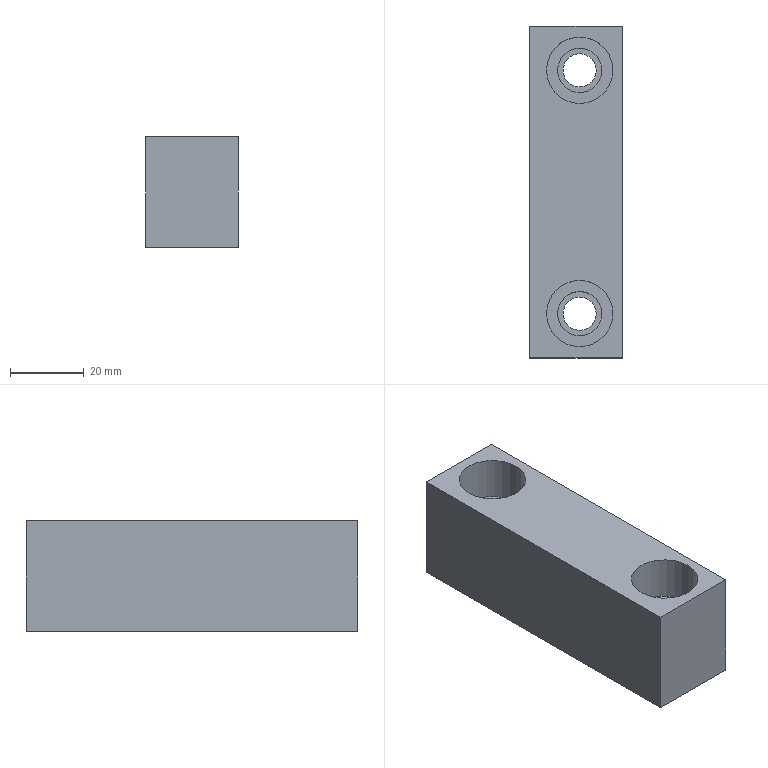Part | STEP file | solid 22 | 1 solid | 16 faces | box 25 x 90 x 30.004 mm | volume 57330 mm3 | plane 10 | cylinder 6 | commonest cylinder face diameters 9 x2 12 x2 18 x2